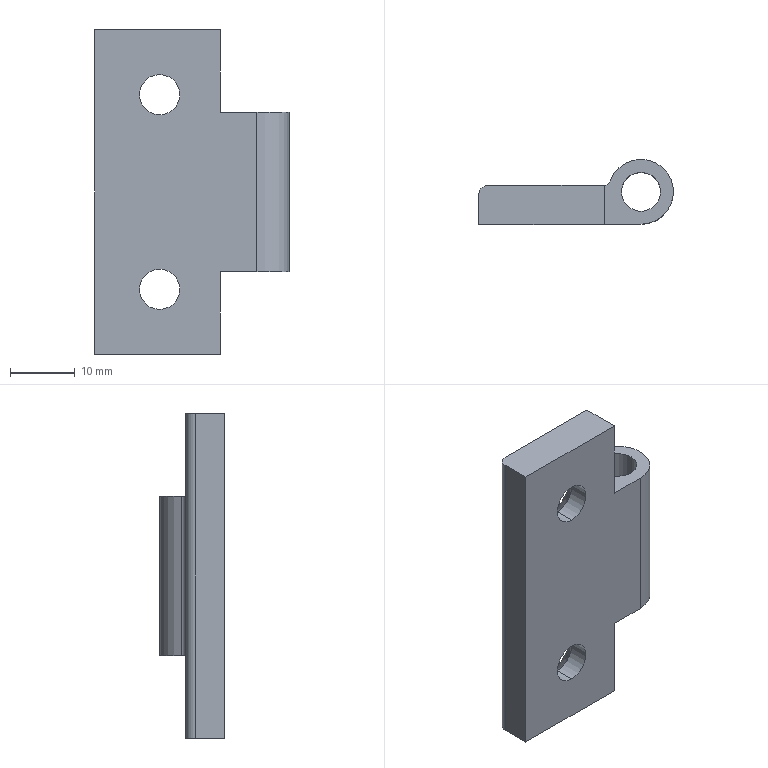Part | STEP file | 750038563 | 1 solid | 22 faces | box 30 x 10 x 50 mm | volume 6670 mm3 | cylinder 9 | plane 9 | cone 4 | commonest cylinder face diameters 6.2 x4 6 x2 2 x1 3 x1 10 x1
STEP:
#1=CARTESIAN_POINT('',(-15.,0.,-11.9));
#2=VERTEX_POINT('',#1);
#3=CARTESIAN_POINT('',(-15.,0.,-18.1));
#4=VERTEX_POINT('',#3);
#5=CARTESIAN_POINT('',(-15.,0.,-15.));
#6=DIRECTION('',(0.,-1.,0.));
#7=DIRECTION('',(0.,0.,1.));
#8=AXIS2_PLACEMENT_3D('',#5,#6,#7);
#9=CIRCLE('',#8,3.1);
#10=EDGE_CURVE('',#2,#4,#9,.T.);
#11=ORIENTED_EDGE('',*,*,#10,.T.);
#12=CARTESIAN_POINT('',(-15.,3.1,-18.1));
#13=VERTEX_POINT('',#12);
#14=CARTESIAN_POINT('',(-15.,-54994.,-18.1));
#15=DIRECTION('',(0.,1.,0.));
#16=VECTOR('',#15,1000.);
#17=LINE('',#14,#16);
#18=EDGE_CURVE('',#4,#13,#17,.T.);
#19=ORIENTED_EDGE('',*,*,#18,.T.);
#20=CARTESIAN_POINT('',(-15.,3.1,-11.9));
#21=VERTEX_POINT('',#20);
#22=CARTESIAN_POINT('',(-15.,3.1,-15.));
#23=DIRECTION('',(0.,-1.,0.));
#24=DIRECTION('',(0.,0.,1.));
#25=AXIS2_PLACEMENT_3D('',#22,#23,#24);
#26=CIRCLE('',#25,3.1);
#27=EDGE_CURVE('',#21,#13,#26,.T.);
#28=ORIENTED_EDGE('',*,*,#27,.F.);
#29=CARTESIAN_POINT('',(-15.,-54994.,-11.9));
#30=DIRECTION('',(0.,1.,0.));
#31=VECTOR('',#30,1000.);
#32=LINE('',#29,#31);
#33=EDGE_CURVE('',#2,#21,#32,.T.);
#34=ORIENTED_EDGE('',*,*,#33,.F.);
#35=EDGE_LOOP('',(#11,#19,#28,#34));
#36=FACE_OUTER_BOUND('',#35,.T.);
#37=CARTESIAN_POINT('',(-15.,-54994.,-15.));
#38=DIRECTION('',(0.,1.,0.));
#39=DIRECTION('',(0.,0.,1.));
#40=AXIS2_PLACEMENT_3D('',#37,#38,#39);
#41=CYLINDRICAL_SURFACE('',#40,3.1);
#42=ADVANCED_FACE('',(#36),#41,.F.);
#43=CARTESIAN_POINT('',(-15.,0.,18.1));
#44=VERTEX_POINT('',#43);
#45=CARTESIAN_POINT('',(-15.,0.,11.9));
#46=VERTEX_POINT('',#45);
#47=CARTESIAN_POINT('',(-15.,0.,15.));
#48=DIRECTION('',(0.,-1.,0.));
#49=DIRECTION('',(0.,0.,1.));
#50=AXIS2_PLACEMENT_3D('',#47,#48,#49);
#51=CIRCLE('',#50,3.1);
#52=EDGE_CURVE('',#44,#46,#51,.T.);
#53=ORIENTED_EDGE('',*,*,#52,.T.);
#54=CARTESIAN_POINT('',(-15.,3.1,11.9));
#55=VERTEX_POINT('',#54);
#56=CARTESIAN_POINT('',(-15.,-54994.,11.9));
#57=DIRECTION('',(0.,1.,0.));
#58=VECTOR('',#57,1000.);
#59=LINE('',#56,#58);
#60=EDGE_CURVE('',#46,#55,#59,.T.);
#61=ORIENTED_EDGE('',*,*,#60,.T.);
#62=CARTESIAN_POINT('',(-15.,3.1,18.1));
#63=VERTEX_POINT('',#62);
#64=CARTESIAN_POINT('',(-15.,3.1,15.));
#65=DIRECTION('',(0.,-1.,0.));
#66=DIRECTION('',(0.,0.,1.));
#67=AXIS2_PLACEMENT_3D('',#64,#65,#66);
#68=CIRCLE('',#67,3.1);
#69=EDGE_CURVE('',#63,#55,#68,.T.);
#70=ORIENTED_EDGE('',*,*,#69,.F.);
#71=CARTESIAN_POINT('',(-15.,-54994.,18.1));
#72=DIRECTION('',(0.,1.,0.));
#73=VECTOR('',#72,1000.);
#74=LINE('',#71,#73);
#75=EDGE_CURVE('',#44,#63,#74,.T.);
#76=ORIENTED_EDGE('',*,*,#75,.F.);
#77=EDGE_LOOP('',(#53,#61,#70,#76));
#78=FACE_OUTER_BOUND('',#77,.T.);
#79=CARTESIAN_POINT('',(-15.,-54994.,15.));
#80=DIRECTION('',(0.,1.,0.));
#81=DIRECTION('',(0.,0.,1.));
#82=AXIS2_PLACEMENT_3D('',#79,#80,#81);
#83=CYLINDRICAL_SURFACE('',#82,3.1);
#84=ADVANCED_FACE('',(#78),#83,.F.);
#85=CARTESIAN_POINT('',(3.,5.,12.3));
#86=VERTEX_POINT('',#85);
#87=CARTESIAN_POINT('',(-3.,5.,12.3));
#88=VERTEX_POINT('',#87);
#89=CARTESIAN_POINT('',(0.,5.,12.3));
#90=DIRECTION('',(0.,0.,-1.));
#91=DIRECTION('',(-1.,0.,0.));
#92=AXIS2_PLACEMENT_3D('',#89,#90,#91);
#93=CIRCLE('',#92,3.);
#94=EDGE_CURVE('',#86,#88,#93,.T.);
#95=ORIENTED_EDGE('',*,*,#94,.F.);
#96=CARTESIAN_POINT('',(3.,5.,-12.3));
#97=VERTEX_POINT('',#96);
#98=CARTESIAN_POINT('',(3.,5.,25.));
#99=DIRECTION('',(0.,0.,-1.));
#100=VECTOR('',#99,1000.);
#101=LINE('',#98,#100);
#102=EDGE_CURVE('',#86,#97,#101,.T.);
#103=ORIENTED_EDGE('',*,*,#102,.T.);
#104=CARTESIAN_POINT('',(-3.,5.,-12.3));
#105=VERTEX_POINT('',#104);
#106=CARTESIAN_POINT('',(0.,5.,-12.3));
#107=DIRECTION('',(0.,0.,1.));
#108=DIRECTION('',(-1.,0.,0.));
#109=AXIS2_PLACEMENT_3D('',#106,#107,#108);
#110=CIRCLE('',#109,3.);
#111=EDGE_CURVE('',#105,#97,#110,.T.);
#112=ORIENTED_EDGE('',*,*,#111,.F.);
#113=CARTESIAN_POINT('',(-3.,5.,25.));
#114=DIRECTION('',(0.,0.,-1.));
#115=VECTOR('',#114,1000.);
#116=LINE('',#113,#115);
#117=EDGE_CURVE('',#88,#105,#116,.T.);
#118=ORIENTED_EDGE('',*,*,#117,.F.);
#119=EDGE_LOOP('',(#95,#103,#112,#118));
#120=FACE_OUTER_BOUND('',#119,.T.);
#121=CARTESIAN_POINT('',(0.,5.,25.));
#122=DIRECTION('',(0.,0.,-1.));
#123=DIRECTION('',(-1.,0.,0.));
#124=AXIS2_PLACEMENT_3D('',#121,#122,#123);
#125=CYLINDRICAL_SURFACE('',#124,3.);
#126=ADVANCED_FACE('',(#120),#125,.F.);
#127=ORIENTED_EDGE('',*,*,#27,.T.);
#128=CARTESIAN_POINT('',(-15.,6.,-21.));
#129=VERTEX_POINT('',#128);
#130=CARTESIAN_POINT('',(-15.,6.,-21.));
#131=DIRECTION('',(0.,0.7071,-0.7071));
#132=VECTOR('',#131,1000.);
#133=LINE('',#130,#132);
#134=EDGE_CURVE('',#13,#129,#133,.T.);
#135=ORIENTED_EDGE('',*,*,#134,.T.);
#136=CARTESIAN_POINT('',(-15.,6.,-9.));
#137=VERTEX_POINT('',#136);
#138=CARTESIAN_POINT('',(-15.,6.,-15.));
#139=DIRECTION('',(0.,1.,0.));
#140=DIRECTION('',(0.,0.,1.));
#141=AXIS2_PLACEMENT_3D('',#138,#139,#140);
#142=CIRCLE('',#141,6.);
#143=EDGE_CURVE('',#129,#137,#142,.T.);
#144=ORIENTED_EDGE('',*,*,#143,.T.);
#145=CARTESIAN_POINT('',(-15.,6.,-9.));
#146=DIRECTION('',(0.,0.7071,0.7071));
#147=VECTOR('',#146,1000.);
#148=LINE('',#145,#147);
#149=EDGE_CURVE('',#21,#137,#148,.T.);
#150=ORIENTED_EDGE('',*,*,#149,.F.);
#151=EDGE_LOOP('',(#127,#135,#144,#150));
#152=FACE_OUTER_BOUND('',#151,.T.);
#153=CARTESIAN_POINT('',(-15.,6.,-15.));
#154=DIRECTION('',(0.,1.,0.));
#155=DIRECTION('',(0.,0.,1.));
#156=AXIS2_PLACEMENT_3D('',#153,#154,#155);
#157=CONICAL_SURFACE('',#156,6.,0.7854);
#158=ADVANCED_FACE('',(#152),#157,.F.);
#159=ORIENTED_EDGE('',*,*,#69,.T.);
#160=CARTESIAN_POINT('',(-15.,6.,9.));
#161=VERTEX_POINT('',#160);
#162=CARTESIAN_POINT('',(-15.,6.,9.));
#163=DIRECTION('',(0.,0.7071,-0.7071));
#164=VECTOR('',#163,1000.);
#165=LINE('',#162,#164);
#166=EDGE_CURVE('',#55,#161,#165,.T.);
#167=ORIENTED_EDGE('',*,*,#166,.T.);
#168=CARTESIAN_POINT('',(-15.,6.,21.));
#169=VERTEX_POINT('',#168);
#170=CARTESIAN_POINT('',(-15.,6.,15.));
#171=DIRECTION('',(0.,1.,0.));
#172=DIRECTION('',(0.,0.,1.));
#173=AXIS2_PLACEMENT_3D('',#170,#171,#172);
#174=CIRCLE('',#173,6.);
#175=EDGE_CURVE('',#161,#169,#174,.T.);
#176=ORIENTED_EDGE('',*,*,#175,.T.);
#177=CARTESIAN_POINT('',(-15.,6.,21.));
#178=DIRECTION('',(0.,0.7071,0.7071));
#179=VECTOR('',#178,1000.);
#180=LINE('',#177,#179);
#181=EDGE_CURVE('',#63,#169,#180,.T.);
#182=ORIENTED_EDGE('',*,*,#181,.F.);
#183=EDGE_LOOP('',(#159,#167,#176,#182));
#184=FACE_OUTER_BOUND('',#183,.T.);
#185=CARTESIAN_POINT('',(-15.,6.,15.));
#186=DIRECTION('',(0.,1.,0.));
#187=DIRECTION('',(0.,0.,1.));
#188=AXIS2_PLACEMENT_3D('',#185,#186,#187);
#189=CONICAL_SURFACE('',#188,6.,0.7854);
#190=ADVANCED_FACE('',(#184),#189,.F.);
#191=CARTESIAN_POINT('',(-25.,0.,25.));
#192=VERTEX_POINT('',#191);
#193=CARTESIAN_POINT('',(-5.657,0.,25.));
#194=VERTEX_POINT('',#193);
#195=CARTESIAN_POINT('',(-25.,0.,25.));
#196=DIRECTION('',(1.,0.,0.));
#197=VECTOR('',#196,1000.);
#198=LINE('',#195,#197);
#199=EDGE_CURVE('',#192,#194,#198,.T.);
#200=ORIENTED_EDGE('',*,*,#199,.F.);
#201=CARTESIAN_POINT('',(-25.,0.,-25.));
#202=VERTEX_POINT('',#201);
#203=CARTESIAN_POINT('',(-25.,0.,25.));
#204=DIRECTION('',(0.,0.,1.));
#205=VECTOR('',#204,1000.);
#206=LINE('',#203,#205);
#207=EDGE_CURVE('',#202,#192,#206,.T.);
#208=ORIENTED_EDGE('',*,*,#207,.F.);
#209=CARTESIAN_POINT('',(-5.657,0.,-25.));
#210=VERTEX_POINT('',#209);
#211=CARTESIAN_POINT('',(-25.,0.,-25.));
#212=DIRECTION('',(-1.,0.,0.));
#213=VECTOR('',#212,1000.);
#214=LINE('',#211,#213);
#215=EDGE_CURVE('',#210,#202,#214,.T.);
#216=ORIENTED_EDGE('',*,*,#215,.F.);
#217=CARTESIAN_POINT('',(-5.657,0.,-12.3));
#218=VERTEX_POINT('',#217);
#219=CARTESIAN_POINT('',(-5.657,0.,25.));
#220=DIRECTION('',(0.,0.,-1.));
#221=VECTOR('',#220,1000.);
#222=LINE('',#219,#221);
#223=EDGE_CURVE('',#218,#210,#222,.T.);
#224=ORIENTED_EDGE('',*,*,#223,.F.);
#225=CARTESIAN_POINT('',(0.,0.,-12.3));
#226=VERTEX_POINT('',#225);
#227=CARTESIAN_POINT('',(-25.,0.,-12.3));
#228=DIRECTION('',(-1.,0.,0.));
#229=VECTOR('',#228,1000.);
#230=LINE('',#227,#229);
#231=EDGE_CURVE('',#226,#218,#230,.T.);
#232=ORIENTED_EDGE('',*,*,#231,.F.);
#233=CARTESIAN_POINT('',(0.,0.,12.3));
#234=VERTEX_POINT('',#233);
#235=CARTESIAN_POINT('',(0.,0.,25.));
#236=DIRECTION('',(0.,0.,-1.));
#237=VECTOR('',#236,1000.);
#238=LINE('',#235,#237);
#239=EDGE_CURVE('',#234,#226,#238,.T.);
#240=ORIENTED_EDGE('',*,*,#239,.F.);
#241=CARTESIAN_POINT('',(-5.657,0.,12.3));
#242=VERTEX_POINT('',#241);
#243=CARTESIAN_POINT('',(-25.,0.,12.3));
#244=DIRECTION('',(1.,0.,0.));
#245=VECTOR('',#244,1000.);
#246=LINE('',#243,#245);
#247=EDGE_CURVE('',#242,#234,#246,.T.);
#248=ORIENTED_EDGE('',*,*,#247,.F.);
#249=CARTESIAN_POINT('',(-5.657,0.,25.));
#250=DIRECTION('',(0.,0.,-1.));
#251=VECTOR('',#250,1000.);
#252=LINE('',#249,#251);
#253=EDGE_CURVE('',#194,#242,#252,.T.);
#254=ORIENTED_EDGE('',*,*,#253,.F.);
#255=EDGE_LOOP('',(#200,#208,#216,#224,#232,#240,#248,#254));
#256=FACE_OUTER_BOUND('',#255,.T.);
#257=ORIENTED_EDGE('',*,*,#10,.F.);
#258=CARTESIAN_POINT('',(-15.,0.,-15.));
#259=DIRECTION('',(0.,-1.,0.));
#260=DIRECTION('',(0.,0.,1.));
#261=AXIS2_PLACEMENT_3D('',#258,#259,#260);
#262=CIRCLE('',#261,3.1);
#263=EDGE_CURVE('',#4,#2,#262,.T.);
#264=ORIENTED_EDGE('',*,*,#263,.F.);
#265=EDGE_LOOP('',(#257,#264));
#266=FACE_BOUND('',#265,.T.);
#267=ORIENTED_EDGE('',*,*,#52,.F.);
#268=CARTESIAN_POINT('',(-15.,0.,15.));
#269=DIRECTION('',(0.,-1.,0.));
#270=DIRECTION('',(0.,0.,1.));
#271=AXIS2_PLACEMENT_3D('',#268,#269,#270);
#272=CIRCLE('',#271,3.1);
#273=EDGE_CURVE('',#46,#44,#272,.T.);
#274=ORIENTED_EDGE('',*,*,#273,.F.);
#275=EDGE_LOOP('',(#267,#274));
#276=FACE_BOUND('',#275,.T.);
#277=CARTESIAN_POINT('',(-25.,0.,25.));
#278=DIRECTION('',(0.,1.,0.));
#279=DIRECTION('',(-1.,0.,0.));
#280=AXIS2_PLACEMENT_3D('',#277,#278,#279);
#281=PLANE('',#280);
#282=ADVANCED_FACE('',(#256,#266,#276),#281,.F.);
#283=CARTESIAN_POINT('',(-5.657,6.,12.3));
#284=VERTEX_POINT('',#283);
#285=CARTESIAN_POINT('',(-5.657,6.,25.));
#286=VERTEX_POINT('',#285);
#287=CARTESIAN_POINT('',(-5.657,6.,12.3));
#288=DIRECTION('',(0.,0.,1.));
#289=VECTOR('',#288,1000.);
#290=LINE('',#287,#289);
#291=EDGE_CURVE('',#284,#286,#290,.T.);
#292=ORIENTED_EDGE('',*,*,#291,.T.);
#293=CARTESIAN_POINT('',(-5.657,31.,25.));
#294=DIRECTION('',(0.,-1.,0.));
#295=VECTOR('',#294,1000.);
#296=LINE('',#293,#295);
#297=EDGE_CURVE('',#286,#194,#296,.T.);
#298=ORIENTED_EDGE('',*,*,#297,.T.);
#299=ORIENTED_EDGE('',*,*,#253,.T.);
#300=CARTESIAN_POINT('',(-5.657,31.,12.3));
#301=DIRECTION('',(0.,1.,0.));
#302=VECTOR('',#301,1000.);
#303=LINE('',#300,#302);
#304=EDGE_CURVE('',#242,#284,#303,.T.);
#305=ORIENTED_EDGE('',*,*,#304,.T.);
#306=EDGE_LOOP('',(#292,#298,#299,#305));
#307=FACE_OUTER_BOUND('',#306,.T.);
#308=CARTESIAN_POINT('',(-5.657,31.,12.3));
#309=DIRECTION('',(1.,0.,0.));
#310=DIRECTION('',(0.,0.,-1.));
#311=AXIS2_PLACEMENT_3D('',#308,#309,#310);
#312=PLANE('',#311);
#313=ADVANCED_FACE('',(#307),#312,.T.);
#314=CARTESIAN_POINT('',(-25.,4.5,25.));
#315=VERTEX_POINT('',#314);
#316=CARTESIAN_POINT('',(-25.,5.,25.));
#317=DIRECTION('',(0.,-1.,0.));
#318=VECTOR('',#317,1000.);
#319=LINE('',#316,#318);
#320=EDGE_CURVE('',#315,#192,#319,.T.);
#321=ORIENTED_EDGE('',*,*,#320,.T.);
#322=ORIENTED_EDGE('',*,*,#199,.T.);
#323=ORIENTED_EDGE('',*,*,#297,.F.);
#324=CARTESIAN_POINT('',(-23.5,6.,25.));
#325=VERTEX_POINT('',#324);
#326=CARTESIAN_POINT('',(0.,6.,25.));
#327=DIRECTION('',(-1.,0.,0.));
#328=VECTOR('',#327,1000.);
#329=LINE('',#326,#328);
#330=EDGE_CURVE('',#286,#325,#329,.T.);
#331=ORIENTED_EDGE('',*,*,#330,.T.);
#332=CARTESIAN_POINT('',(-23.5,4.5,25.));
#333=DIRECTION('',(0.,0.,1.));
#334=DIRECTION('',(-1.,0.,0.));
#335=AXIS2_PLACEMENT_3D('',#332,#333,#334);
#336=CIRCLE('',#335,1.5);
#337=EDGE_CURVE('',#325,#315,#336,.T.);
#338=ORIENTED_EDGE('',*,*,#337,.T.);
#339=EDGE_LOOP('',(#321,#322,#323,#331,#338));
#340=FACE_OUTER_BOUND('',#339,.T.);
#341=CARTESIAN_POINT('',(0.,5.,25.));
#342=DIRECTION('',(0.,0.,1.));
#343=DIRECTION('',(1.,0.,0.));
#344=AXIS2_PLACEMENT_3D('',#341,#342,#343);
#345=PLANE('',#344);
#346=ADVANCED_FACE('',(#340),#345,.T.);
#347=ORIENTED_EDGE('',*,*,#207,.T.);
#348=ORIENTED_EDGE('',*,*,#320,.F.);
#349=CARTESIAN_POINT('',(-25.,4.5,-25.));
#350=VERTEX_POINT('',#349);
#351=CARTESIAN_POINT('',(-25.,4.5,25.));
#352=DIRECTION('',(0.,0.,1.));
#353=VECTOR('',#352,1000.);
#354=LINE('',#351,#353);
#355=EDGE_CURVE('',#350,#315,#354,.T.);
#356=ORIENTED_EDGE('',*,*,#355,.F.);
#357=CARTESIAN_POINT('',(-25.,4.5,-25.));
#358=DIRECTION('',(0.,1.,0.));
#359=VECTOR('',#358,1000.);
#360=LINE('',#357,#359);
#361=EDGE_CURVE('',#202,#350,#360,.T.);
#362=ORIENTED_EDGE('',*,*,#361,.F.);
#363=EDGE_LOOP('',(#347,#348,#356,#362));
#364=FACE_OUTER_BOUND('',#363,.T.);
#365=CARTESIAN_POINT('',(-25.,4.5,25.));
#366=DIRECTION('',(1.,0.,0.));
#367=DIRECTION('',(0.,0.,-1.));
#368=AXIS2_PLACEMENT_3D('',#365,#366,#367);
#369=PLANE('',#368);
#370=ADVANCED_FACE('',(#364),#369,.F.);
#371=CARTESIAN_POINT('',(-5.657,6.,-25.));
#372=VERTEX_POINT('',#371);
#373=CARTESIAN_POINT('',(-5.657,5.,-25.));
#374=DIRECTION('',(0.,1.,0.));
#375=VECTOR('',#374,1000.);
#376=LINE('',#373,#375);
#377=EDGE_CURVE('',#210,#372,#376,.T.);
#378=ORIENTED_EDGE('',*,*,#377,.F.);
#379=ORIENTED_EDGE('',*,*,#215,.T.);
#380=ORIENTED_EDGE('',*,*,#361,.T.);
#381=CARTESIAN_POINT('',(-23.5,6.,-25.));
#382=VERTEX_POINT('',#381);
#383=CARTESIAN_POINT('',(-23.5,4.5,-25.));
#384=DIRECTION('',(0.,0.,1.));
#385=DIRECTION('',(-1.,0.,0.));
#386=AXIS2_PLACEMENT_3D('',#383,#384,#385);
#387=CIRCLE('',#386,1.5);
#388=EDGE_CURVE('',#382,#350,#387,.T.);
#389=ORIENTED_EDGE('',*,*,#388,.F.);
#390=CARTESIAN_POINT('',(0.,6.,-25.));
#391=DIRECTION('',(-1.,0.,0.));
#392=VECTOR('',#391,1000.);
#393=LINE('',#390,#392);
#394=EDGE_CURVE('',#372,#382,#393,.T.);
#395=ORIENTED_EDGE('',*,*,#394,.F.);
#396=EDGE_LOOP('',(#378,#379,#380,#389,#395));
#397=FACE_OUTER_BOUND('',#396,.T.);
#398=CARTESIAN_POINT('',(0.,5.,-25.));
#399=DIRECTION('',(0.,0.,1.));
#400=DIRECTION('',(1.,0.,0.));
#401=AXIS2_PLACEMENT_3D('',#398,#399,#400);
#402=PLANE('',#401);
#403=ADVANCED_FACE('',(#397),#402,.F.);
#404=CARTESIAN_POINT('',(-5.657,6.,-12.3));
#405=VERTEX_POINT('',#404);
#406=CARTESIAN_POINT('',(-5.657,6.,-25.));
#407=DIRECTION('',(0.,0.,1.));
#408=VECTOR('',#407,1000.);
#409=LINE('',#406,#408);
#410=EDGE_CURVE('',#372,#405,#409,.T.);
#411=ORIENTED_EDGE('',*,*,#410,.T.);
#412=CARTESIAN_POINT('',(-5.657,31.,-12.3));
#413=DIRECTION('',(0.,-1.,0.));
#414=VECTOR('',#413,1000.);
#415=LINE('',#412,#414);
#416=EDGE_CURVE('',#405,#218,#415,.T.);
#417=ORIENTED_EDGE('',*,*,#416,.T.);
#418=ORIENTED_EDGE('',*,*,#223,.T.);
#419=ORIENTED_EDGE('',*,*,#377,.T.);
#420=EDGE_LOOP('',(#411,#417,#418,#419));
#421=FACE_OUTER_BOUND('',#420,.T.);
#422=CARTESIAN_POINT('',(-5.657,31.,-25.));
#423=DIRECTION('',(1.,0.,0.));
#424=DIRECTION('',(0.,0.,-1.));
#425=AXIS2_PLACEMENT_3D('',#422,#423,#424);
#426=PLANE('',#425);
#427=ADVANCED_FACE('',(#421),#426,.T.);
#428=CARTESIAN_POINT('',(-4.714,6.667,-12.3));
#429=VERTEX_POINT('',#428);
#430=CARTESIAN_POINT('',(-5.657,7.,-12.3));
#431=DIRECTION('',(0.,0.,1.));
#432=DIRECTION('',(-1.,0.,0.));
#433=AXIS2_PLACEMENT_3D('',#430,#431,#432);
#434=CIRCLE('',#433,1.);
#435=EDGE_CURVE('',#405,#429,#434,.T.);
#436=ORIENTED_EDGE('',*,*,#435,.T.);
#437=CARTESIAN_POINT('',(0.,5.,-12.3));
#438=DIRECTION('',(0.,0.,-1.));
#439=DIRECTION('',(-1.,0.,0.));
#440=AXIS2_PLACEMENT_3D('',#437,#438,#439);
#441=CIRCLE('',#440,5.);
#442=EDGE_CURVE('',#429,#226,#441,.T.);
#443=ORIENTED_EDGE('',*,*,#442,.T.);
#444=ORIENTED_EDGE('',*,*,#231,.T.);
#445=ORIENTED_EDGE('',*,*,#416,.F.);
#446=EDGE_LOOP('',(#436,#443,#444,#445));
#447=FACE_OUTER_BOUND('',#446,.T.);
#448=ORIENTED_EDGE('',*,*,#111,.T.);
#449=CARTESIAN_POINT('',(0.,5.,-12.3));
#450=DIRECTION('',(0.,0.,1.));
#451=DIRECTION('',(-1.,0.,0.));
#452=AXIS2_PLACEMENT_3D('',#449,#450,#451);
#453=CIRCLE('',#452,3.);
#454=EDGE_CURVE('',#97,#105,#453,.T.);
#455=ORIENTED_EDGE('',*,*,#454,.T.);
#456=EDGE_LOOP('',(#448,#455));
#457=FACE_BOUND('',#456,.T.);
#458=CARTESIAN_POINT('',(-5.657,31.,-12.3));
#459=DIRECTION('',(0.,0.,-1.));
#460=DIRECTION('',(-1.,0.,0.));
#461=AXIS2_PLACEMENT_3D('',#458,#459,#460);
#462=PLANE('',#461);
#463=ADVANCED_FACE('',(#447,#457),#462,.T.);
#464=ORIENTED_EDGE('',*,*,#239,.T.);
#465=ORIENTED_EDGE('',*,*,#442,.F.);
#466=CARTESIAN_POINT('',(-4.714,6.667,12.3));
#467=VERTEX_POINT('',#466);
#468=CARTESIAN_POINT('',(-4.714,6.667,25.));
#469=DIRECTION('',(0.,0.,1.));
#470=VECTOR('',#469,1000.);
#471=LINE('',#468,#470);
#472=EDGE_CURVE('',#429,#467,#471,.T.);
#473=ORIENTED_EDGE('',*,*,#472,.T.);
#474=CARTESIAN_POINT('',(0.,5.,12.3));
#475=DIRECTION('',(0.,0.,-1.));
#476=DIRECTION('',(-1.,0.,0.));
#477=AXIS2_PLACEMENT_3D('',#474,#475,#476);
#478=CIRCLE('',#477,5.);
#479=EDGE_CURVE('',#467,#234,#478,.T.);
#480=ORIENTED_EDGE('',*,*,#479,.T.);
#481=EDGE_LOOP('',(#464,#465,#473,#480));
#482=FACE_OUTER_BOUND('',#481,.T.);
#483=CARTESIAN_POINT('',(0.,5.,25.));
#484=DIRECTION('',(0.,0.,-1.));
#485=DIRECTION('',(-1.,0.,0.));
#486=AXIS2_PLACEMENT_3D('',#483,#484,#485);
#487=CYLINDRICAL_SURFACE('',#486,5.);
#488=ADVANCED_FACE('',(#482),#487,.T.);
#489=CARTESIAN_POINT('',(-5.657,7.,12.3));
#490=DIRECTION('',(0.,0.,-1.));
#491=DIRECTION('',(-1.,0.,0.));
#492=AXIS2_PLACEMENT_3D('',#489,#490,#491);
#493=CIRCLE('',#492,1.);
#494=EDGE_CURVE('',#467,#284,#493,.T.);
#495=ORIENTED_EDGE('',*,*,#494,.T.);
#496=ORIENTED_EDGE('',*,*,#304,.F.);
#497=ORIENTED_EDGE('',*,*,#247,.T.);
#498=ORIENTED_EDGE('',*,*,#479,.F.);
#499=EDGE_LOOP('',(#495,#496,#497,#498));
#500=FACE_OUTER_BOUND('',#499,.T.);
#501=CARTESIAN_POINT('',(0.,5.,12.3));
#502=DIRECTION('',(0.,0.,-1.));
#503=DIRECTION('',(-1.,0.,0.));
#504=AXIS2_PLACEMENT_3D('',#501,#502,#503);
#505=CIRCLE('',#504,3.);
#506=EDGE_CURVE('',#88,#86,#505,.T.);
#507=ORIENTED_EDGE('',*,*,#506,.T.);
#508=ORIENTED_EDGE('',*,*,#94,.T.);
#509=EDGE_LOOP('',(#507,#508));
#510=FACE_BOUND('',#509,.T.);
#511=CARTESIAN_POINT('',(5.,31.,12.3));
#512=DIRECTION('',(0.,0.,1.));
#513=DIRECTION('',(1.,0.,0.));
#514=AXIS2_PLACEMENT_3D('',#511,#512,#513);
#515=PLANE('',#514);
#516=ADVANCED_FACE('',(#500,#510),#515,.T.);
#517=ORIENTED_EDGE('',*,*,#18,.F.);
#518=ORIENTED_EDGE('',*,*,#263,.T.);
#519=ORIENTED_EDGE('',*,*,#33,.T.);
#520=CARTESIAN_POINT('',(-15.,3.1,-15.));
#521=DIRECTION('',(0.,-1.,0.));
#522=DIRECTION('',(0.,0.,1.));
#523=AXIS2_PLACEMENT_3D('',#520,#521,#522);
#524=CIRCLE('',#523,3.1);
#525=EDGE_CURVE('',#13,#21,#524,.T.);
#526=ORIENTED_EDGE('',*,*,#525,.F.);
#527=EDGE_LOOP('',(#517,#518,#519,#526));
#528=FACE_OUTER_BOUND('',#527,.T.);
#529=CARTESIAN_POINT('',(-15.,-54994.,-15.));
#530=DIRECTION('',(0.,1.,0.));
#531=DIRECTION('',(0.,0.,1.));
#532=AXIS2_PLACEMENT_3D('',#529,#530,#531);
#533=CYLINDRICAL_SURFACE('',#532,3.1);
#534=ADVANCED_FACE('',(#528),#533,.F.);
#535=ORIENTED_EDGE('',*,*,#60,.F.);
#536=ORIENTED_EDGE('',*,*,#273,.T.);
#537=ORIENTED_EDGE('',*,*,#75,.T.);
#538=CARTESIAN_POINT('',(-15.,3.1,15.));
#539=DIRECTION('',(0.,-1.,0.));
#540=DIRECTION('',(0.,0.,1.));
#541=AXIS2_PLACEMENT_3D('',#538,#539,#540);
#542=CIRCLE('',#541,3.1);
#543=EDGE_CURVE('',#55,#63,#542,.T.);
#544=ORIENTED_EDGE('',*,*,#543,.F.);
#545=EDGE_LOOP('',(#535,#536,#537,#544));
#546=FACE_OUTER_BOUND('',#545,.T.);
#547=CARTESIAN_POINT('',(-15.,-54994.,15.));
#548=DIRECTION('',(0.,1.,0.));
#549=DIRECTION('',(0.,0.,1.));
#550=AXIS2_PLACEMENT_3D('',#547,#548,#549);
#551=CYLINDRICAL_SURFACE('',#550,3.1);
#552=ADVANCED_FACE('',(#546),#551,.F.);
#553=CARTESIAN_POINT('',(-23.5,6.,25.));
#554=DIRECTION('',(0.,0.,-1.));
#555=VECTOR('',#554,1000.);
#556=LINE('',#553,#555);
#557=EDGE_CURVE('',#325,#382,#556,.T.);
#558=ORIENTED_EDGE('',*,*,#557,.F.);
#559=ORIENTED_EDGE('',*,*,#330,.F.);
#560=ORIENTED_EDGE('',*,*,#291,.F.);
#561=CARTESIAN_POINT('',(-5.657,6.,25.));
#562=DIRECTION('',(0.,0.,1.));
#563=VECTOR('',#562,1000.);
#564=LINE('',#561,#563);
#565=EDGE_CURVE('',#405,#284,#564,.T.);
#566=ORIENTED_EDGE('',*,*,#565,.F.);
#567=ORIENTED_EDGE('',*,*,#410,.F.);
#568=ORIENTED_EDGE('',*,*,#394,.T.);
#569=EDGE_LOOP('',(#558,#559,#560,#566,#567,#568));
#570=FACE_OUTER_BOUND('',#569,.T.);
#571=CARTESIAN_POINT('',(-15.,6.,-15.));
#572=DIRECTION('',(0.,1.,0.));
#573=DIRECTION('',(0.,0.,1.));
#574=AXIS2_PLACEMENT_3D('',#571,#572,#573);
#575=CIRCLE('',#574,6.);
#576=EDGE_CURVE('',#137,#129,#575,.T.);
#577=ORIENTED_EDGE('',*,*,#576,.F.);
#578=ORIENTED_EDGE('',*,*,#143,.F.);
#579=EDGE_LOOP('',(#577,#578));
#580=FACE_BOUND('',#579,.T.);
#581=CARTESIAN_POINT('',(-15.,6.,15.));
#582=DIRECTION('',(0.,1.,0.));
#583=DIRECTION('',(0.,0.,1.));
#584=AXIS2_PLACEMENT_3D('',#581,#582,#583);
#585=CIRCLE('',#584,6.);
#586=EDGE_CURVE('',#169,#161,#585,.T.);
#587=ORIENTED_EDGE('',*,*,#586,.F.);
#588=ORIENTED_EDGE('',*,*,#175,.F.);
#589=EDGE_LOOP('',(#587,#588));
#590=FACE_BOUND('',#589,.T.);
#591=CARTESIAN_POINT('',(-5.657,6.,25.));
#592=DIRECTION('',(0.,-1.,0.));
#593=DIRECTION('',(1.,0.,0.));
#594=AXIS2_PLACEMENT_3D('',#591,#592,#593);
#595=PLANE('',#594);
#596=ADVANCED_FACE('',(#570,#580,#590),#595,.F.);
#597=ORIENTED_EDGE('',*,*,#337,.F.);
#598=ORIENTED_EDGE('',*,*,#557,.T.);
#599=ORIENTED_EDGE('',*,*,#388,.T.);
#600=ORIENTED_EDGE('',*,*,#355,.T.);
#601=EDGE_LOOP('',(#597,#598,#599,#600));
#602=FACE_OUTER_BOUND('',#601,.T.);
#603=CARTESIAN_POINT('',(-23.5,4.5,25.));
#604=DIRECTION('',(0.,0.,-1.));
#605=DIRECTION('',(-1.,0.,0.));
#606=AXIS2_PLACEMENT_3D('',#603,#604,#605);
#607=CYLINDRICAL_SURFACE('',#606,1.5);
#608=ADVANCED_FACE('',(#602),#607,.T.);
#609=ORIENTED_EDGE('',*,*,#102,.F.);
#610=ORIENTED_EDGE('',*,*,#506,.F.);
#611=ORIENTED_EDGE('',*,*,#117,.T.);
#612=ORIENTED_EDGE('',*,*,#454,.F.);
#613=EDGE_LOOP('',(#609,#610,#611,#612));
#614=FACE_OUTER_BOUND('',#613,.T.);
#615=CARTESIAN_POINT('',(0.,5.,25.));
#616=DIRECTION('',(0.,0.,-1.));
#617=DIRECTION('',(-1.,0.,0.));
#618=AXIS2_PLACEMENT_3D('',#615,#616,#617);
#619=CYLINDRICAL_SURFACE('',#618,3.);
#620=ADVANCED_FACE('',(#614),#619,.F.);
#621=ORIENTED_EDGE('',*,*,#472,.F.);
#622=ORIENTED_EDGE('',*,*,#435,.F.);
#623=ORIENTED_EDGE('',*,*,#565,.T.);
#624=ORIENTED_EDGE('',*,*,#494,.F.);
#625=EDGE_LOOP('',(#621,#622,#623,#624));
#626=FACE_OUTER_BOUND('',#625,.T.);
#627=CARTESIAN_POINT('',(-5.657,7.,25.));
#628=DIRECTION('',(0.,0.,-1.));
#629=DIRECTION('',(-1.,0.,0.));
#630=AXIS2_PLACEMENT_3D('',#627,#628,#629);
#631=CYLINDRICAL_SURFACE('',#630,1.);
#632=ADVANCED_FACE('',(#626),#631,.F.);
#633=ORIENTED_EDGE('',*,*,#134,.F.);
#634=ORIENTED_EDGE('',*,*,#525,.T.);
#635=ORIENTED_EDGE('',*,*,#149,.T.);
#636=ORIENTED_EDGE('',*,*,#576,.T.);
#637=EDGE_LOOP('',(#633,#634,#635,#636));
#638=FACE_OUTER_BOUND('',#637,.T.);
#639=CARTESIAN_POINT('',(-15.,6.,-15.));
#640=DIRECTION('',(0.,1.,0.));
#641=DIRECTION('',(0.,0.,1.));
#642=AXIS2_PLACEMENT_3D('',#639,#640,#641);
#643=CONICAL_SURFACE('',#642,6.,0.7854);
#644=ADVANCED_FACE('',(#638),#643,.F.);
#645=ORIENTED_EDGE('',*,*,#166,.F.);
#646=ORIENTED_EDGE('',*,*,#543,.T.);
#647=ORIENTED_EDGE('',*,*,#181,.T.);
#648=ORIENTED_EDGE('',*,*,#586,.T.);
#649=EDGE_LOOP('',(#645,#646,#647,#648));
#650=FACE_OUTER_BOUND('',#649,.T.);
#651=CARTESIAN_POINT('',(-15.,6.,15.));
#652=DIRECTION('',(0.,1.,0.));
#653=DIRECTION('',(0.,0.,1.));
#654=AXIS2_PLACEMENT_3D('',#651,#652,#653);
#655=CONICAL_SURFACE('',#654,6.,0.7854);
#656=ADVANCED_FACE('',(#650),#655,.F.);
#657=CLOSED_SHELL('',(#42,#84,#126,#158,#190,#282,#313,#346,#370,#403,#427,#463,#488,#516,#534,#552,#596,#608,#620,#632,#644,#656));
#658=MANIFOLD_SOLID_BREP('',#657);
#659=CARTESIAN_POINT('',(0.,0.,0.));
#660=DIRECTION('',(0.,0.,1.));
#661=DIRECTION('',(1.,0.,0.));
#662=AXIS2_PLACEMENT_3D('',#659,#660,#661);
#663=(LENGTH_UNIT()NAMED_UNIT(*)SI_UNIT(.MILLI.,.METRE.));
#664=UNCERTAINTY_MEASURE_WITH_UNIT(LENGTH_MEASURE(0.00001),#663,'','');
#665=(NAMED_UNIT(*)PLANE_ANGLE_UNIT()SI_UNIT($,.RADIAN.));
#666=(NAMED_UNIT(*)SI_UNIT($,.STERADIAN.)SOLID_ANGLE_UNIT());
#667=(GEOMETRIC_REPRESENTATION_CONTEXT(3)GLOBAL_UNCERTAINTY_ASSIGNED_CONTEXT((#664))GLOBAL_UNIT_ASSIGNED_CONTEXT((#663,#665,#666))REPRESENTATION_CONTEXT('',''));
#668=ADVANCED_BREP_SHAPE_REPRESENTATION('',(#658,#662),#667);